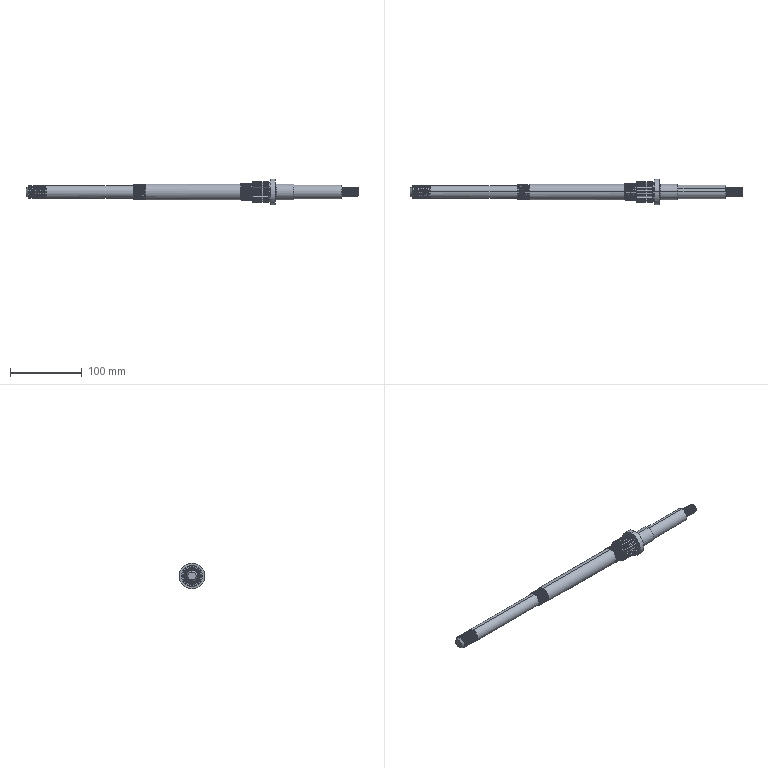Part | STEP file | Completa.sldasm-Part-112_Valor predeterminado | 1 solid | 463 faces | box 464 x 36 x 36 mm | volume 151077 mm3 | cylinder 346 | plane 82 | spline 22 | torus 8 | cone 5 | commonest cylinder face diameters 16 x53 17 x52 11 x45 12 x45 22.1 x31 23 x31